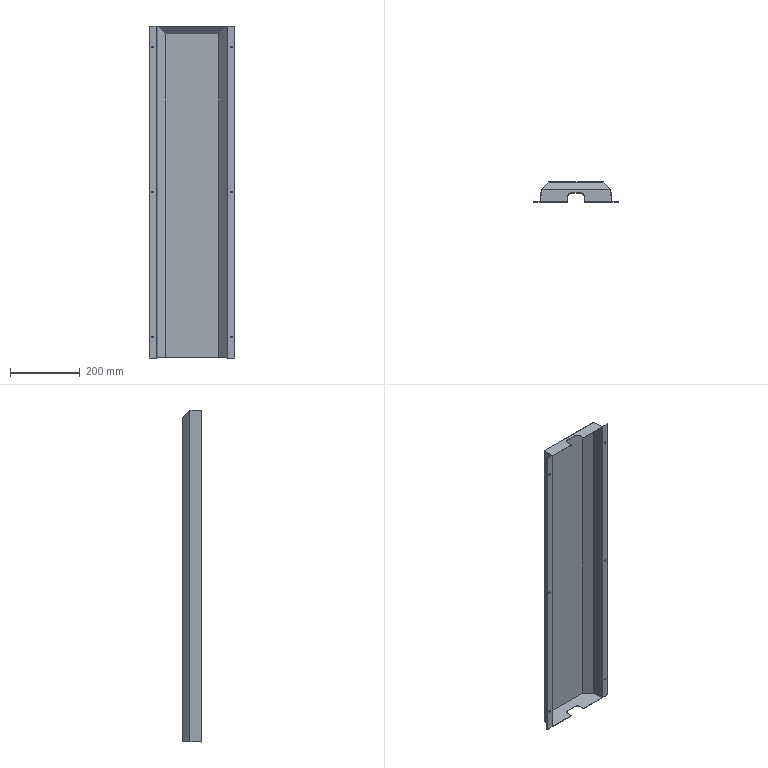Part | STEP file | 101000007774 | 3 solids | 52 faces | box 245 x 56 x 950 mm | volume 323951 mm3 | plane 36 | cylinder 16 | commonest cylinder face diameters 5.2 x12 25 x4